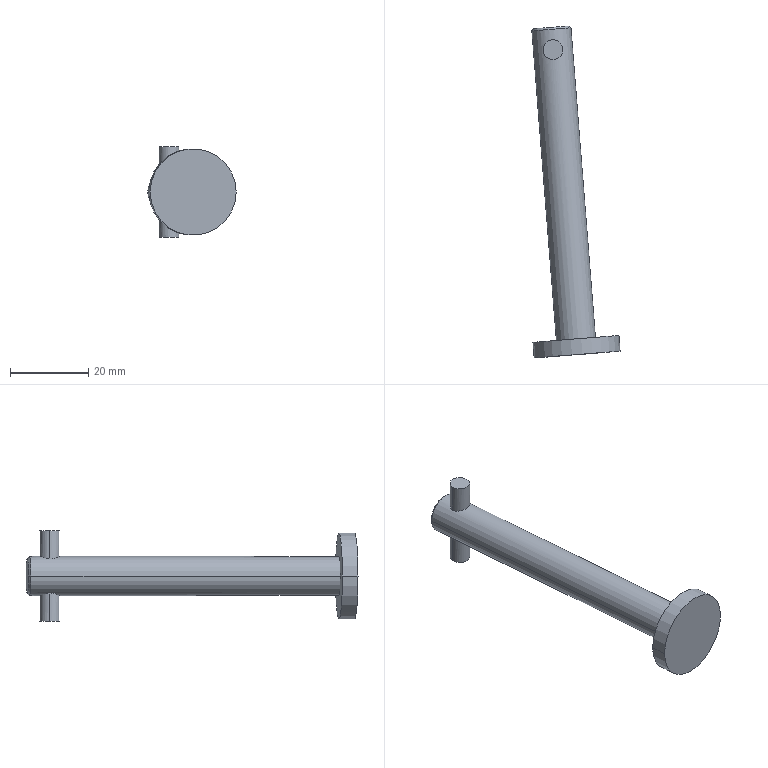Part | STEP file | Sceond_200_APVM0 -2 | 1 solid | 15 faces | box 22.523 x 84.663 x 23 mm | volume 8038 mm3 | cylinder 8 | plane 5 | cone 2 | commonest cylinder face diameters 5 x4 10 x2 22 x2